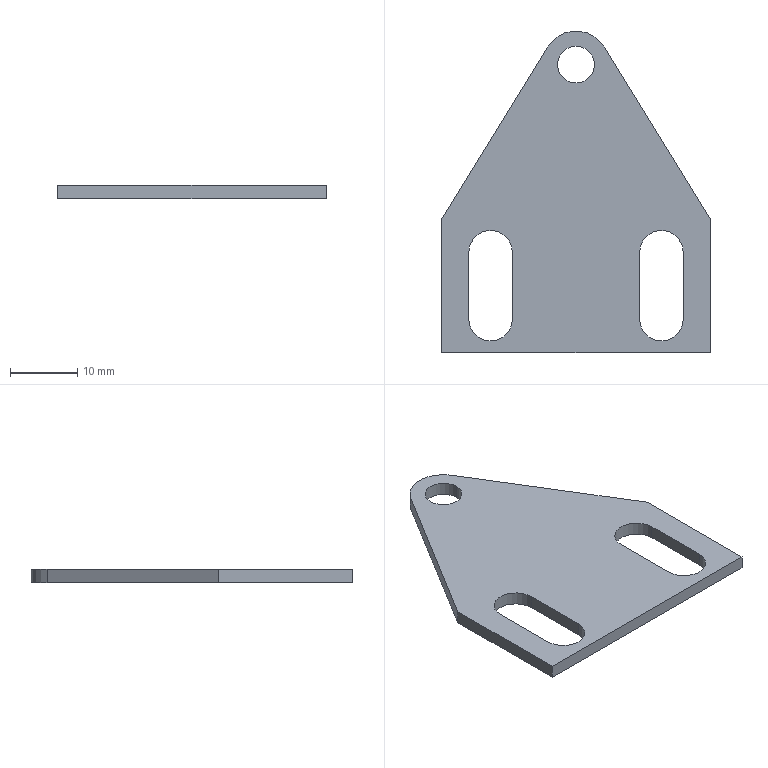Part | STEP file | Door catch sheet metal | 1 solid | 18 faces | box 40 x 48 x 2 mm | volume 2431 mm3 | plane 11 | cylinder 7 | commonest cylinder face diameters 6.5 x4 5.5 x2 10 x1
STEP:
#1=CARTESIAN_POINT('',(0.,0.,0.));
#2=DIRECTION('',(0.,0.,1.));
#3=DIRECTION('',(1.,0.,0.));
#4=AXIS2_PLACEMENT_3D('',#1,#2,#3);
#5=CARTESIAN_POINT('',(-2.75,19.,2.));
#6=VERTEX_POINT('',#5);
#7=CARTESIAN_POINT('',(-2.75,19.,0.));
#8=VERTEX_POINT('',#7);
#9=CARTESIAN_POINT('',(-2.75,19.,2.));
#10=DIRECTION('',(0.,0.,-1.));
#11=VECTOR('',#10,1.);
#12=LINE('',#9,#11);
#13=CARTESIAN_POINT('',(0.,19.,2.));
#14=DIRECTION('',(0.,0.,-1.));
#15=DIRECTION('',(-1.,0.,0.));
#16=AXIS2_PLACEMENT_3D('',#13,#14,#15);
#17=CYLINDRICAL_SURFACE('',#16,2.75);
#18=CARTESIAN_POINT('',(6.283,0.));
#19=DIRECTION('',(0.,1.));
#20=VECTOR('',#19,1.);
#21=LINE('',#18,#20);
#22=(GEOMETRIC_REPRESENTATION_CONTEXT(2)PARAMETRIC_REPRESENTATION_CONTEXT()REPRESENTATION_CONTEXT('',''));
#23=DEFINITIONAL_REPRESENTATION('',(#21),#22);
#24=PCURVE('',#17,#23);
#25=CARTESIAN_POINT('',(0.,19.,2.));
#26=DIRECTION('',(0.,0.,-1.));
#27=DIRECTION('',(-1.,0.,0.));
#28=AXIS2_PLACEMENT_3D('',#25,#26,#27);
#29=CYLINDRICAL_SURFACE('',#28,2.75);
#30=CARTESIAN_POINT('',(0.,0.));
#31=DIRECTION('',(0.,1.));
#32=VECTOR('',#31,1.);
#33=LINE('',#30,#32);
#34=(GEOMETRIC_REPRESENTATION_CONTEXT(2)PARAMETRIC_REPRESENTATION_CONTEXT()REPRESENTATION_CONTEXT('',''));
#35=DEFINITIONAL_REPRESENTATION('',(#33),#34);
#36=PCURVE('',#29,#35);
#37=SURFACE_CURVE('',#12,(#24,#36),.PCURVE_S1.);
#38=EDGE_CURVE('',#6,#8,#37,.T.);
#39=ORIENTED_EDGE('',*,*,#38,.T.);
#40=CARTESIAN_POINT('',(2.75,19.,0.));
#41=VERTEX_POINT('',#40);
#42=CARTESIAN_POINT('',(0.,19.,0.));
#43=DIRECTION('',(0.,0.,1.));
#44=DIRECTION('',(1.,0.,0.));
#45=AXIS2_PLACEMENT_3D('',#42,#43,#44);
#46=CIRCLE('',#45,2.75);
#47=CARTESIAN_POINT('',(9.425,2.));
#48=DIRECTION('',(-1.,0.));
#49=VECTOR('',#48,1.);
#50=LINE('',#47,#49);
#51=(GEOMETRIC_REPRESENTATION_CONTEXT(2)PARAMETRIC_REPRESENTATION_CONTEXT()REPRESENTATION_CONTEXT('',''));
#52=DEFINITIONAL_REPRESENTATION('',(#50),#51);
#53=PCURVE('',#17,#52);
#54=CARTESIAN_POINT('',(0.,0.,0.));
#55=DIRECTION('',(0.,0.,1.));
#56=DIRECTION('',(1.,0.,0.));
#57=AXIS2_PLACEMENT_3D('',#54,#55,#56);
#58=PLANE('',#57);
#59=CARTESIAN_POINT('',(0.,19.));
#60=DIRECTION('',(1.,0.));
#61=AXIS2_PLACEMENT_2D('',#59,#60);
#62=CIRCLE('',#61,2.75);
#63=(GEOMETRIC_REPRESENTATION_CONTEXT(2)PARAMETRIC_REPRESENTATION_CONTEXT()REPRESENTATION_CONTEXT('',''));
#64=DEFINITIONAL_REPRESENTATION('',(#62),#63);
#65=PCURVE('',#58,#64);
#66=SURFACE_CURVE('',#46,(#53,#65),.PCURVE_S1.);
#67=EDGE_CURVE('',#8,#41,#66,.T.);
#68=ORIENTED_EDGE('',*,*,#67,.T.);
#69=CARTESIAN_POINT('',(2.75,19.,2.));
#70=VERTEX_POINT('',#69);
#71=CARTESIAN_POINT('',(2.75,19.,2.));
#72=DIRECTION('',(0.,0.,-1.));
#73=VECTOR('',#72,1.);
#74=LINE('',#71,#73);
#75=CARTESIAN_POINT('',(3.142,0.));
#76=DIRECTION('',(0.,1.));
#77=VECTOR('',#76,1.);
#78=LINE('',#75,#77);
#79=(GEOMETRIC_REPRESENTATION_CONTEXT(2)PARAMETRIC_REPRESENTATION_CONTEXT()REPRESENTATION_CONTEXT('',''));
#80=DEFINITIONAL_REPRESENTATION('',(#78),#79);
#81=PCURVE('',#17,#80);
#82=CARTESIAN_POINT('',(3.142,0.));
#83=DIRECTION('',(0.,1.));
#84=VECTOR('',#83,1.);
#85=LINE('',#82,#84);
#86=(GEOMETRIC_REPRESENTATION_CONTEXT(2)PARAMETRIC_REPRESENTATION_CONTEXT()REPRESENTATION_CONTEXT('',''));
#87=DEFINITIONAL_REPRESENTATION('',(#85),#86);
#88=PCURVE('',#29,#87);
#89=SURFACE_CURVE('',#74,(#81,#88),.PCURVE_S1.);
#90=EDGE_CURVE('',#70,#41,#89,.T.);
#91=ORIENTED_EDGE('',*,*,#90,.F.);
#92=CARTESIAN_POINT('',(0.,19.,2.));
#93=DIRECTION('',(0.,0.,1.));
#94=DIRECTION('',(1.,0.,0.));
#95=AXIS2_PLACEMENT_3D('',#92,#93,#94);
#96=CIRCLE('',#95,2.75);
#97=CARTESIAN_POINT('',(9.425,0.));
#98=DIRECTION('',(-1.,0.));
#99=VECTOR('',#98,1.);
#100=LINE('',#97,#99);
#101=(GEOMETRIC_REPRESENTATION_CONTEXT(2)PARAMETRIC_REPRESENTATION_CONTEXT()REPRESENTATION_CONTEXT('',''));
#102=DEFINITIONAL_REPRESENTATION('',(#100),#101);
#103=PCURVE('',#17,#102);
#104=CARTESIAN_POINT('',(0.,0.,2.));
#105=DIRECTION('',(0.,0.,1.));
#106=DIRECTION('',(1.,0.,0.));
#107=AXIS2_PLACEMENT_3D('',#104,#105,#106);
#108=PLANE('',#107);
#109=CARTESIAN_POINT('',(0.,19.));
#110=DIRECTION('',(1.,0.));
#111=AXIS2_PLACEMENT_2D('',#109,#110);
#112=CIRCLE('',#111,2.75);
#113=(GEOMETRIC_REPRESENTATION_CONTEXT(2)PARAMETRIC_REPRESENTATION_CONTEXT()REPRESENTATION_CONTEXT('',''));
#114=DEFINITIONAL_REPRESENTATION('',(#112),#113);
#115=PCURVE('',#108,#114);
#116=SURFACE_CURVE('',#96,(#103,#115),.PCURVE_S1.);
#117=EDGE_CURVE('',#6,#70,#116,.T.);
#118=ORIENTED_EDGE('',*,*,#117,.F.);
#119=EDGE_LOOP('',(#39,#68,#91,#118));
#120=FACE_BOUND('',#119,.F.);
#121=ADVANCED_FACE('',(#120),#17,.F.);
#122=CARTESIAN_POINT('',(4.26,21.618,0.));
#123=VERTEX_POINT('',#122);
#124=CARTESIAN_POINT('',(20.,-4.,0.));
#125=VERTEX_POINT('',#124);
#126=CARTESIAN_POINT('',(12.735,7.825,0.));
#127=DIRECTION('',(0.5235,-0.852,0.));
#128=VECTOR('',#127,1.);
#129=LINE('',#126,#128);
#130=CARTESIAN_POINT('',(12.735,7.825,2.));
#131=DIRECTION('',(0.852,0.5235,0.));
#132=DIRECTION('',(-0.5235,0.852,0.));
#133=AXIS2_PLACEMENT_3D('',#130,#131,#132);
#134=PLANE('',#133);
#135=CARTESIAN_POINT('',(0.,-2.));
#136=DIRECTION('',(-1.,0.));
#137=VECTOR('',#136,1.);
#138=LINE('',#135,#137);
#139=(GEOMETRIC_REPRESENTATION_CONTEXT(2)PARAMETRIC_REPRESENTATION_CONTEXT()REPRESENTATION_CONTEXT('',''));
#140=DEFINITIONAL_REPRESENTATION('',(#138),#139);
#141=PCURVE('',#134,#140);
#142=CARTESIAN_POINT('',(12.735,7.825));
#143=DIRECTION('',(0.5235,-0.852));
#144=VECTOR('',#143,1.);
#145=LINE('',#142,#144);
#146=(GEOMETRIC_REPRESENTATION_CONTEXT(2)PARAMETRIC_REPRESENTATION_CONTEXT()REPRESENTATION_CONTEXT('',''));
#147=DEFINITIONAL_REPRESENTATION('',(#145),#146);
#148=PCURVE('',#58,#147);
#149=SURFACE_CURVE('',#129,(#141,#148),.PCURVE_S1.);
#150=EDGE_CURVE('',#123,#125,#149,.T.);
#151=ORIENTED_EDGE('',*,*,#150,.F.);
#152=CARTESIAN_POINT('',(4.26,21.618,2.));
#153=VERTEX_POINT('',#152);
#154=CARTESIAN_POINT('',(4.26,21.618,2.));
#155=DIRECTION('',(0.,0.,-1.));
#156=VECTOR('',#155,1.);
#157=LINE('',#154,#156);
#158=CARTESIAN_POINT('',(16.188,0.));
#159=DIRECTION('',(0.,-1.));
#160=VECTOR('',#159,1.);
#161=LINE('',#158,#160);
#162=(GEOMETRIC_REPRESENTATION_CONTEXT(2)PARAMETRIC_REPRESENTATION_CONTEXT()REPRESENTATION_CONTEXT('',''));
#163=DEFINITIONAL_REPRESENTATION('',(#161),#162);
#164=PCURVE('',#134,#163);
#165=CARTESIAN_POINT('',(0.,19.,2.));
#166=DIRECTION('',(0.,0.,-1.));
#167=DIRECTION('',(-1.,0.,0.));
#168=AXIS2_PLACEMENT_3D('',#165,#166,#167);
#169=CYLINDRICAL_SURFACE('',#168,5.);
#170=CARTESIAN_POINT('',(2.591,0.));
#171=DIRECTION('',(0.,1.));
#172=VECTOR('',#171,1.);
#173=LINE('',#170,#172);
#174=(GEOMETRIC_REPRESENTATION_CONTEXT(2)PARAMETRIC_REPRESENTATION_CONTEXT()REPRESENTATION_CONTEXT('',''));
#175=DEFINITIONAL_REPRESENTATION('',(#173),#174);
#176=PCURVE('',#169,#175);
#177=SURFACE_CURVE('',#157,(#164,#176),.PCURVE_S1.);
#178=EDGE_CURVE('',#153,#123,#177,.T.);
#179=ORIENTED_EDGE('',*,*,#178,.F.);
#180=CARTESIAN_POINT('',(20.,-4.,2.));
#181=VERTEX_POINT('',#180);
#182=CARTESIAN_POINT('',(12.735,7.825,2.));
#183=DIRECTION('',(0.5235,-0.852,0.));
#184=VECTOR('',#183,1.);
#185=LINE('',#182,#184);
#186=CARTESIAN_POINT('',(0.,0.));
#187=DIRECTION('',(-1.,0.));
#188=VECTOR('',#187,1.);
#189=LINE('',#186,#188);
#190=(GEOMETRIC_REPRESENTATION_CONTEXT(2)PARAMETRIC_REPRESENTATION_CONTEXT()REPRESENTATION_CONTEXT('',''));
#191=DEFINITIONAL_REPRESENTATION('',(#189),#190);
#192=PCURVE('',#134,#191);
#193=CARTESIAN_POINT('',(12.735,7.825));
#194=DIRECTION('',(0.5235,-0.852));
#195=VECTOR('',#194,1.);
#196=LINE('',#193,#195);
#197=(GEOMETRIC_REPRESENTATION_CONTEXT(2)PARAMETRIC_REPRESENTATION_CONTEXT()REPRESENTATION_CONTEXT('',''));
#198=DEFINITIONAL_REPRESENTATION('',(#196),#197);
#199=PCURVE('',#108,#198);
#200=SURFACE_CURVE('',#185,(#192,#199),.PCURVE_S1.);
#201=EDGE_CURVE('',#153,#181,#200,.T.);
#202=ORIENTED_EDGE('',*,*,#201,.T.);
#203=CARTESIAN_POINT('',(20.,-4.,2.));
#204=DIRECTION('',(0.,0.,-1.));
#205=VECTOR('',#204,1.);
#206=LINE('',#203,#205);
#207=CARTESIAN_POINT('',(-13.878,0.));
#208=DIRECTION('',(0.,-1.));
#209=VECTOR('',#208,1.);
#210=LINE('',#207,#209);
#211=(GEOMETRIC_REPRESENTATION_CONTEXT(2)PARAMETRIC_REPRESENTATION_CONTEXT()REPRESENTATION_CONTEXT('',''));
#212=DEFINITIONAL_REPRESENTATION('',(#210),#211);
#213=PCURVE('',#134,#212);
#214=CARTESIAN_POINT('',(20.,0.,2.));
#215=DIRECTION('',(1.,0.,0.));
#216=DIRECTION('',(0.,1.,0.));
#217=AXIS2_PLACEMENT_3D('',#214,#215,#216);
#218=PLANE('',#217);
#219=CARTESIAN_POINT('',(-4.,0.));
#220=DIRECTION('',(0.,-1.));
#221=VECTOR('',#220,1.);
#222=LINE('',#219,#221);
#223=(GEOMETRIC_REPRESENTATION_CONTEXT(2)PARAMETRIC_REPRESENTATION_CONTEXT()REPRESENTATION_CONTEXT('',''));
#224=DEFINITIONAL_REPRESENTATION('',(#222),#223);
#225=PCURVE('',#218,#224);
#226=SURFACE_CURVE('',#206,(#213,#225),.PCURVE_S1.);
#227=EDGE_CURVE('',#181,#125,#226,.T.);
#228=ORIENTED_EDGE('',*,*,#227,.T.);
#229=EDGE_LOOP('',(#151,#179,#202,#228));
#230=FACE_BOUND('',#229,.T.);
#231=ADVANCED_FACE('',(#230),#134,.T.);
#232=CARTESIAN_POINT('',(-4.26,21.618,0.));
#233=VERTEX_POINT('',#232);
#234=CARTESIAN_POINT('',(0.,19.,0.));
#235=DIRECTION('',(0.,0.,1.));
#236=DIRECTION('',(1.,0.,0.));
#237=AXIS2_PLACEMENT_3D('',#234,#235,#236);
#238=CIRCLE('',#237,5.);
#239=CARTESIAN_POINT('',(3.142,2.));
#240=DIRECTION('',(-1.,0.));
#241=VECTOR('',#240,1.);
#242=LINE('',#239,#241);
#243=(GEOMETRIC_REPRESENTATION_CONTEXT(2)PARAMETRIC_REPRESENTATION_CONTEXT()REPRESENTATION_CONTEXT('',''));
#244=DEFINITIONAL_REPRESENTATION('',(#242),#243);
#245=PCURVE('',#169,#244);
#246=CARTESIAN_POINT('',(0.,19.));
#247=DIRECTION('',(1.,0.));
#248=AXIS2_PLACEMENT_2D('',#246,#247);
#249=CIRCLE('',#248,5.);
#250=(GEOMETRIC_REPRESENTATION_CONTEXT(2)PARAMETRIC_REPRESENTATION_CONTEXT()REPRESENTATION_CONTEXT('',''));
#251=DEFINITIONAL_REPRESENTATION('',(#249),#250);
#252=PCURVE('',#58,#251);
#253=SURFACE_CURVE('',#238,(#245,#252),.PCURVE_S1.);
#254=EDGE_CURVE('',#123,#233,#253,.T.);
#255=ORIENTED_EDGE('',*,*,#254,.T.);
#256=CARTESIAN_POINT('',(-4.26,21.618,2.));
#257=VERTEX_POINT('',#256);
#258=CARTESIAN_POINT('',(-4.26,21.618,2.));
#259=DIRECTION('',(0.,0.,-1.));
#260=VECTOR('',#259,1.);
#261=LINE('',#258,#260);
#262=CARTESIAN_POINT('',(0.551,0.));
#263=DIRECTION('',(0.,1.));
#264=VECTOR('',#263,1.);
#265=LINE('',#262,#264);
#266=(GEOMETRIC_REPRESENTATION_CONTEXT(2)PARAMETRIC_REPRESENTATION_CONTEXT()REPRESENTATION_CONTEXT('',''));
#267=DEFINITIONAL_REPRESENTATION('',(#265),#266);
#268=PCURVE('',#169,#267);
#269=CARTESIAN_POINT('',(-12.735,7.825,2.));
#270=DIRECTION('',(0.852,-0.5235,0.));
#271=DIRECTION('',(0.5235,0.852,0.));
#272=AXIS2_PLACEMENT_3D('',#269,#270,#271);
#273=PLANE('',#272);
#274=CARTESIAN_POINT('',(16.188,0.));
#275=DIRECTION('',(0.,-1.));
#276=VECTOR('',#275,1.);
#277=LINE('',#274,#276);
#278=(GEOMETRIC_REPRESENTATION_CONTEXT(2)PARAMETRIC_REPRESENTATION_CONTEXT()REPRESENTATION_CONTEXT('',''));
#279=DEFINITIONAL_REPRESENTATION('',(#277),#278);
#280=PCURVE('',#273,#279);
#281=SURFACE_CURVE('',#261,(#268,#280),.PCURVE_S1.);
#282=EDGE_CURVE('',#257,#233,#281,.T.);
#283=ORIENTED_EDGE('',*,*,#282,.F.);
#284=CARTESIAN_POINT('',(0.,19.,2.));
#285=DIRECTION('',(0.,0.,1.));
#286=DIRECTION('',(1.,0.,0.));
#287=AXIS2_PLACEMENT_3D('',#284,#285,#286);
#288=CIRCLE('',#287,5.);
#289=CARTESIAN_POINT('',(3.142,0.));
#290=DIRECTION('',(-1.,0.));
#291=VECTOR('',#290,1.);
#292=LINE('',#289,#291);
#293=(GEOMETRIC_REPRESENTATION_CONTEXT(2)PARAMETRIC_REPRESENTATION_CONTEXT()REPRESENTATION_CONTEXT('',''));
#294=DEFINITIONAL_REPRESENTATION('',(#292),#293);
#295=PCURVE('',#169,#294);
#296=CARTESIAN_POINT('',(0.,19.));
#297=DIRECTION('',(1.,0.));
#298=AXIS2_PLACEMENT_2D('',#296,#297);
#299=CIRCLE('',#298,5.);
#300=(GEOMETRIC_REPRESENTATION_CONTEXT(2)PARAMETRIC_REPRESENTATION_CONTEXT()REPRESENTATION_CONTEXT('',''));
#301=DEFINITIONAL_REPRESENTATION('',(#299),#300);
#302=PCURVE('',#108,#301);
#303=SURFACE_CURVE('',#288,(#295,#302),.PCURVE_S1.);
#304=EDGE_CURVE('',#153,#257,#303,.T.);
#305=ORIENTED_EDGE('',*,*,#304,.F.);
#306=ORIENTED_EDGE('',*,*,#178,.T.);
#307=EDGE_LOOP('',(#255,#283,#305,#306));
#308=FACE_BOUND('',#307,.T.);
#309=ADVANCED_FACE('',(#308),#169,.T.);
#310=CARTESIAN_POINT('',(-20.,-4.,0.));
#311=VERTEX_POINT('',#310);
#312=CARTESIAN_POINT('',(-12.735,7.825,0.));
#313=DIRECTION('',(-0.5235,-0.852,0.));
#314=VECTOR('',#313,1.);
#315=LINE('',#312,#314);
#316=CARTESIAN_POINT('',(0.,-2.));
#317=DIRECTION('',(-1.,0.));
#318=VECTOR('',#317,1.);
#319=LINE('',#316,#318);
#320=(GEOMETRIC_REPRESENTATION_CONTEXT(2)PARAMETRIC_REPRESENTATION_CONTEXT()REPRESENTATION_CONTEXT('',''));
#321=DEFINITIONAL_REPRESENTATION('',(#319),#320);
#322=PCURVE('',#273,#321);
#323=CARTESIAN_POINT('',(-12.735,7.825));
#324=DIRECTION('',(-0.5235,-0.852));
#325=VECTOR('',#324,1.);
#326=LINE('',#323,#325);
#327=(GEOMETRIC_REPRESENTATION_CONTEXT(2)PARAMETRIC_REPRESENTATION_CONTEXT()REPRESENTATION_CONTEXT('',''));
#328=DEFINITIONAL_REPRESENTATION('',(#326),#327);
#329=PCURVE('',#58,#328);
#330=SURFACE_CURVE('',#315,(#322,#329),.PCURVE_S1.);
#331=EDGE_CURVE('',#233,#311,#330,.T.);
#332=ORIENTED_EDGE('',*,*,#331,.T.);
#333=CARTESIAN_POINT('',(-20.,-4.,2.));
#334=VERTEX_POINT('',#333);
#335=CARTESIAN_POINT('',(-20.,-4.,2.));
#336=DIRECTION('',(0.,0.,-1.));
#337=VECTOR('',#336,1.);
#338=LINE('',#335,#337);
#339=CARTESIAN_POINT('',(-13.878,0.));
#340=DIRECTION('',(0.,-1.));
#341=VECTOR('',#340,1.);
#342=LINE('',#339,#341);
#343=(GEOMETRIC_REPRESENTATION_CONTEXT(2)PARAMETRIC_REPRESENTATION_CONTEXT()REPRESENTATION_CONTEXT('',''));
#344=DEFINITIONAL_REPRESENTATION('',(#342),#343);
#345=PCURVE('',#273,#344);
#346=CARTESIAN_POINT('',(-20.,0.,2.));
#347=DIRECTION('',(1.,0.,0.));
#348=DIRECTION('',(0.,1.,0.));
#349=AXIS2_PLACEMENT_3D('',#346,#347,#348);
#350=PLANE('',#349);
#351=CARTESIAN_POINT('',(-4.,0.));
#352=DIRECTION('',(0.,-1.));
#353=VECTOR('',#352,1.);
#354=LINE('',#351,#353);
#355=(GEOMETRIC_REPRESENTATION_CONTEXT(2)PARAMETRIC_REPRESENTATION_CONTEXT()REPRESENTATION_CONTEXT('',''));
#356=DEFINITIONAL_REPRESENTATION('',(#354),#355);
#357=PCURVE('',#350,#356);
#358=SURFACE_CURVE('',#338,(#345,#357),.PCURVE_S1.);
#359=EDGE_CURVE('',#334,#311,#358,.T.);
#360=ORIENTED_EDGE('',*,*,#359,.F.);
#361=CARTESIAN_POINT('',(-12.735,7.825,2.));
#362=DIRECTION('',(-0.5235,-0.852,0.));
#363=VECTOR('',#362,1.);
#364=LINE('',#361,#363);
#365=CARTESIAN_POINT('',(0.,0.));
#366=DIRECTION('',(-1.,0.));
#367=VECTOR('',#366,1.);
#368=LINE('',#365,#367);
#369=(GEOMETRIC_REPRESENTATION_CONTEXT(2)PARAMETRIC_REPRESENTATION_CONTEXT()REPRESENTATION_CONTEXT('',''));
#370=DEFINITIONAL_REPRESENTATION('',(#368),#369);
#371=PCURVE('',#273,#370);
#372=CARTESIAN_POINT('',(-12.735,7.825));
#373=DIRECTION('',(-0.5235,-0.852));
#374=VECTOR('',#373,1.);
#375=LINE('',#372,#374);
#376=(GEOMETRIC_REPRESENTATION_CONTEXT(2)PARAMETRIC_REPRESENTATION_CONTEXT()REPRESENTATION_CONTEXT('',''));
#377=DEFINITIONAL_REPRESENTATION('',(#375),#376);
#378=PCURVE('',#108,#377);
#379=SURFACE_CURVE('',#364,(#371,#378),.PCURVE_S1.);
#380=EDGE_CURVE('',#257,#334,#379,.T.);
#381=ORIENTED_EDGE('',*,*,#380,.F.);
#382=ORIENTED_EDGE('',*,*,#282,.T.);
#383=EDGE_LOOP('',(#332,#360,#381,#382));
#384=FACE_BOUND('',#383,.T.);
#385=ADVANCED_FACE('',(#384),#273,.F.);
#386=CARTESIAN_POINT('',(-20.,-24.,0.));
#387=VERTEX_POINT('',#386);
#388=CARTESIAN_POINT('',(-20.,0.,0.));
#389=DIRECTION('',(0.,-1.,0.));
#390=VECTOR('',#389,1.);
#391=LINE('',#388,#390);
#392=CARTESIAN_POINT('',(0.,-2.));
#393=DIRECTION('',(-1.,0.));
#394=VECTOR('',#393,1.);
#395=LINE('',#392,#394);
#396=(GEOMETRIC_REPRESENTATION_CONTEXT(2)PARAMETRIC_REPRESENTATION_CONTEXT()REPRESENTATION_CONTEXT('',''));
#397=DEFINITIONAL_REPRESENTATION('',(#395),#396);
#398=PCURVE('',#350,#397);
#399=CARTESIAN_POINT('',(-20.,0.));
#400=DIRECTION('',(0.,-1.));
#401=VECTOR('',#400,1.);
#402=LINE('',#399,#401);
#403=(GEOMETRIC_REPRESENTATION_CONTEXT(2)PARAMETRIC_REPRESENTATION_CONTEXT()REPRESENTATION_CONTEXT('',''));
#404=DEFINITIONAL_REPRESENTATION('',(#402),#403);
#405=PCURVE('',#58,#404);
#406=SURFACE_CURVE('',#391,(#398,#405),.PCURVE_S1.);
#407=EDGE_CURVE('',#311,#387,#406,.T.);
#408=ORIENTED_EDGE('',*,*,#407,.T.);
#409=CARTESIAN_POINT('',(-20.,-24.,2.));
#410=VERTEX_POINT('',#409);
#411=CARTESIAN_POINT('',(-20.,-24.,2.));
#412=DIRECTION('',(0.,0.,-1.));
#413=VECTOR('',#412,1.);
#414=LINE('',#411,#413);
#415=CARTESIAN_POINT('',(-24.,0.));
#416=DIRECTION('',(0.,-1.));
#417=VECTOR('',#416,1.);
#418=LINE('',#415,#417);
#419=(GEOMETRIC_REPRESENTATION_CONTEXT(2)PARAMETRIC_REPRESENTATION_CONTEXT()REPRESENTATION_CONTEXT('',''));
#420=DEFINITIONAL_REPRESENTATION('',(#418),#419);
#421=PCURVE('',#350,#420);
#422=CARTESIAN_POINT('',(0.,-24.,2.));
#423=DIRECTION('',(0.,1.,0.));
#424=DIRECTION('',(0.,0.,1.));
#425=AXIS2_PLACEMENT_3D('',#422,#423,#424);
#426=PLANE('',#425);
#427=CARTESIAN_POINT('',(0.,-20.));
#428=DIRECTION('',(-1.,0.));
#429=VECTOR('',#428,1.);
#430=LINE('',#427,#429);
#431=(GEOMETRIC_REPRESENTATION_CONTEXT(2)PARAMETRIC_REPRESENTATION_CONTEXT()REPRESENTATION_CONTEXT('',''));
#432=DEFINITIONAL_REPRESENTATION('',(#430),#431);
#433=PCURVE('',#426,#432);
#434=SURFACE_CURVE('',#414,(#421,#433),.PCURVE_S1.);
#435=EDGE_CURVE('',#410,#387,#434,.T.);
#436=ORIENTED_EDGE('',*,*,#435,.F.);
#437=CARTESIAN_POINT('',(-20.,0.,2.));
#438=DIRECTION('',(0.,-1.,0.));
#439=VECTOR('',#438,1.);
#440=LINE('',#437,#439);
#441=CARTESIAN_POINT('',(0.,0.));
#442=DIRECTION('',(-1.,0.));
#443=VECTOR('',#442,1.);
#444=LINE('',#441,#443);
#445=(GEOMETRIC_REPRESENTATION_CONTEXT(2)PARAMETRIC_REPRESENTATION_CONTEXT()REPRESENTATION_CONTEXT('',''));
#446=DEFINITIONAL_REPRESENTATION('',(#444),#445);
#447=PCURVE('',#350,#446);
#448=CARTESIAN_POINT('',(-20.,0.));
#449=DIRECTION('',(0.,-1.));
#450=VECTOR('',#449,1.);
#451=LINE('',#448,#450);
#452=(GEOMETRIC_REPRESENTATION_CONTEXT(2)PARAMETRIC_REPRESENTATION_CONTEXT()REPRESENTATION_CONTEXT('',''));
#453=DEFINITIONAL_REPRESENTATION('',(#451),#452);
#454=PCURVE('',#108,#453);
#455=SURFACE_CURVE('',#440,(#447,#454),.PCURVE_S1.);
#456=EDGE_CURVE('',#334,#410,#455,.T.);
#457=ORIENTED_EDGE('',*,*,#456,.F.);
#458=ORIENTED_EDGE('',*,*,#359,.T.);
#459=EDGE_LOOP('',(#408,#436,#457,#458));
#460=FACE_BOUND('',#459,.T.);
#461=ADVANCED_FACE('',(#460),#350,.F.);
#462=CARTESIAN_POINT('',(20.,-24.,0.));
#463=VERTEX_POINT('',#462);
#464=CARTESIAN_POINT('',(0.,-24.,0.));
#465=DIRECTION('',(1.,0.,0.));
#466=VECTOR('',#465,1.);
#467=LINE('',#464,#466);
#468=CARTESIAN_POINT('',(-2.,0.));
#469=DIRECTION('',(0.,1.));
#470=VECTOR('',#469,1.);
#471=LINE('',#468,#470);
#472=(GEOMETRIC_REPRESENTATION_CONTEXT(2)PARAMETRIC_REPRESENTATION_CONTEXT()REPRESENTATION_CONTEXT('',''));
#473=DEFINITIONAL_REPRESENTATION('',(#471),#472);
#474=PCURVE('',#426,#473);
#475=CARTESIAN_POINT('',(0.,-24.));
#476=DIRECTION('',(1.,0.));
#477=VECTOR('',#476,1.);
#478=LINE('',#475,#477);
#479=(GEOMETRIC_REPRESENTATION_CONTEXT(2)PARAMETRIC_REPRESENTATION_CONTEXT()REPRESENTATION_CONTEXT('',''));
#480=DEFINITIONAL_REPRESENTATION('',(#478),#479);
#481=PCURVE('',#58,#480);
#482=SURFACE_CURVE('',#467,(#474,#481),.PCURVE_S1.);
#483=EDGE_CURVE('',#387,#463,#482,.T.);
#484=ORIENTED_EDGE('',*,*,#483,.T.);
#485=CARTESIAN_POINT('',(20.,-24.,2.));
#486=VERTEX_POINT('',#485);
#487=CARTESIAN_POINT('',(20.,-24.,2.));
#488=DIRECTION('',(0.,0.,-1.));
#489=VECTOR('',#488,1.);
#490=LINE('',#487,#489);
#491=CARTESIAN_POINT('',(0.,20.));
#492=DIRECTION('',(-1.,0.));
#493=VECTOR('',#492,1.);
#494=LINE('',#491,#493);
#495=(GEOMETRIC_REPRESENTATION_CONTEXT(2)PARAMETRIC_REPRESENTATION_CONTEXT()REPRESENTATION_CONTEXT('',''));
#496=DEFINITIONAL_REPRESENTATION('',(#494),#495);
#497=PCURVE('',#426,#496);
#498=CARTESIAN_POINT('',(-24.,0.));
#499=DIRECTION('',(0.,-1.));
#500=VECTOR('',#499,1.);
#501=LINE('',#498,#500);
#502=(GEOMETRIC_REPRESENTATION_CONTEXT(2)PARAMETRIC_REPRESENTATION_CONTEXT()REPRESENTATION_CONTEXT('',''));
#503=DEFINITIONAL_REPRESENTATION('',(#501),#502);
#504=PCURVE('',#218,#503);
#505=SURFACE_CURVE('',#490,(#497,#504),.PCURVE_S1.);
#506=EDGE_CURVE('',#486,#463,#505,.T.);
#507=ORIENTED_EDGE('',*,*,#506,.F.);
#508=CARTESIAN_POINT('',(0.,-24.,2.));
#509=DIRECTION('',(1.,0.,0.));
#510=VECTOR('',#509,1.);
#511=LINE('',#508,#510);
#512=CARTESIAN_POINT('',(0.,0.));
#513=DIRECTION('',(0.,1.));
#514=VECTOR('',#513,1.);
#515=LINE('',#512,#514);
#516=(GEOMETRIC_REPRESENTATION_CONTEXT(2)PARAMETRIC_REPRESENTATION_CONTEXT()REPRESENTATION_CONTEXT('',''));
#517=DEFINITIONAL_REPRESENTATION('',(#515),#516);
#518=PCURVE('',#426,#517);
#519=CARTESIAN_POINT('',(0.,-24.));
#520=DIRECTION('',(1.,0.));
#521=VECTOR('',#520,1.);
#522=LINE('',#519,#521);
#523=(GEOMETRIC_REPRESENTATION_CONTEXT(2)PARAMETRIC_REPRESENTATION_CONTEXT()REPRESENTATION_CONTEXT('',''));
#524=DEFINITIONAL_REPRESENTATION('',(#522),#523);
#525=PCURVE('',#108,#524);
#526=SURFACE_CURVE('',#511,(#518,#525),.PCURVE_S1.);
#527=EDGE_CURVE('',#410,#486,#526,.T.);
#528=ORIENTED_EDGE('',*,*,#527,.F.);
#529=ORIENTED_EDGE('',*,*,#435,.T.);
#530=EDGE_LOOP('',(#484,#507,#528,#529));
#531=FACE_BOUND('',#530,.T.);
#532=ADVANCED_FACE('',(#531),#426,.F.);
#533=CARTESIAN_POINT('',(-9.5,-19.,2.));
#534=VERTEX_POINT('',#533);
#535=CARTESIAN_POINT('',(-9.5,-19.,0.));
#536=VERTEX_POINT('',#535);
#537=CARTESIAN_POINT('',(-9.5,-19.,2.));
#538=DIRECTION('',(0.,0.,-1.));
#539=VECTOR('',#538,1.);
#540=LINE('',#537,#539);
#541=CARTESIAN_POINT('',(-12.75,-19.,2.));
#542=DIRECTION('',(0.,0.,-1.));
#543=DIRECTION('',(-1.,0.,0.));
#544=AXIS2_PLACEMENT_3D('',#541,#542,#543);
#545=CYLINDRICAL_SURFACE('',#544,3.25);
#546=CARTESIAN_POINT('',(3.142,0.));
#547=DIRECTION('',(0.,1.));
#548=VECTOR('',#547,1.);
#549=LINE('',#546,#548);
#550=(GEOMETRIC_REPRESENTATION_CONTEXT(2)PARAMETRIC_REPRESENTATION_CONTEXT()REPRESENTATION_CONTEXT('',''));
#551=DEFINITIONAL_REPRESENTATION('',(#549),#550);
#552=PCURVE('',#545,#551);
#553=CARTESIAN_POINT('',(-9.5,0.,2.));
#554=DIRECTION('',(1.,0.,0.));
#555=DIRECTION('',(0.,0.,-1.));
#556=AXIS2_PLACEMENT_3D('',#553,#554,#555);
#557=PLANE('',#556);
#558=CARTESIAN_POINT('',(0.,-19.));
#559=DIRECTION('',(1.,0.));
#560=VECTOR('',#559,1.);
#561=LINE('',#558,#560);
#562=(GEOMETRIC_REPRESENTATION_CONTEXT(2)PARAMETRIC_REPRESENTATION_CONTEXT()REPRESENTATION_CONTEXT('',''));
#563=DEFINITIONAL_REPRESENTATION('',(#561),#562);
#564=PCURVE('',#557,#563);
#565=SURFACE_CURVE('',#540,(#552,#564),.PCURVE_S1.);
#566=EDGE_CURVE('',#534,#536,#565,.T.);
#567=ORIENTED_EDGE('',*,*,#566,.F.);
#568=CARTESIAN_POINT('',(-16.,-19.,2.));
#569=VERTEX_POINT('',#568);
#570=CARTESIAN_POINT('',(-12.75,-19.,2.));
#571=DIRECTION('',(0.,0.,1.));
#572=DIRECTION('',(1.,0.,0.));
#573=AXIS2_PLACEMENT_3D('',#570,#571,#572);
#574=CIRCLE('',#573,3.25);
#575=CARTESIAN_POINT('',(9.425,0.));
#576=DIRECTION('',(-1.,0.));
#577=VECTOR('',#576,1.);
#578=LINE('',#575,#577);
#579=(GEOMETRIC_REPRESENTATION_CONTEXT(2)PARAMETRIC_REPRESENTATION_CONTEXT()REPRESENTATION_CONTEXT('',''));
#580=DEFINITIONAL_REPRESENTATION('',(#578),#579);
#581=PCURVE('',#545,#580);
#582=CARTESIAN_POINT('',(-12.75,-19.));
#583=DIRECTION('',(1.,0.));
#584=AXIS2_PLACEMENT_2D('',#582,#583);
#585=CIRCLE('',#584,3.25);
#586=(GEOMETRIC_REPRESENTATION_CONTEXT(2)PARAMETRIC_REPRESENTATION_CONTEXT()REPRESENTATION_CONTEXT('',''));
#587=DEFINITIONAL_REPRESENTATION('',(#585),#586);
#588=PCURVE('',#108,#587);
#589=SURFACE_CURVE('',#574,(#581,#588),.PCURVE_S1.);
#590=EDGE_CURVE('',#569,#534,#589,.T.);
#591=ORIENTED_EDGE('',*,*,#590,.F.);
#592=CARTESIAN_POINT('',(-16.,-19.,0.));
#593=VERTEX_POINT('',#592);
#594=CARTESIAN_POINT('',(-16.,-19.,2.));
#595=DIRECTION('',(0.,0.,-1.));
#596=VECTOR('',#595,1.);
#597=LINE('',#594,#596);
#598=CARTESIAN_POINT('',(6.283,0.));
#599=DIRECTION('',(0.,1.));
#600=VECTOR('',#599,1.);
#601=LINE('',#598,#600);
#602=(GEOMETRIC_REPRESENTATION_CONTEXT(2)PARAMETRIC_REPRESENTATION_CONTEXT()REPRESENTATION_CONTEXT('',''));
#603=DEFINITIONAL_REPRESENTATION('',(#601),#602);
#604=PCURVE('',#545,#603);
#605=CARTESIAN_POINT('',(-16.,0.,2.));
#606=DIRECTION('',(1.,0.,0.));
#607=DIRECTION('',(0.,0.,-1.));
#608=AXIS2_PLACEMENT_3D('',#605,#606,#607);
#609=PLANE('',#608);
#610=CARTESIAN_POINT('',(0.,-19.));
#611=DIRECTION('',(1.,0.));
#612=VECTOR('',#611,1.);
#613=LINE('',#610,#612);
#614=(GEOMETRIC_REPRESENTATION_CONTEXT(2)PARAMETRIC_REPRESENTATION_CONTEXT()REPRESENTATION_CONTEXT('',''));
#615=DEFINITIONAL_REPRESENTATION('',(#613),#614);
#616=PCURVE('',#609,#615);
#617=SURFACE_CURVE('',#597,(#604,#616),.PCURVE_S1.);
#618=EDGE_CURVE('',#569,#593,#617,.T.);
#619=ORIENTED_EDGE('',*,*,#618,.T.);
#620=CARTESIAN_POINT('',(-12.75,-19.,0.));
#621=DIRECTION('',(0.,0.,1.));
#622=DIRECTION('',(1.,0.,0.));
#623=AXIS2_PLACEMENT_3D('',#620,#621,#622);
#624=CIRCLE('',#623,3.25);
#625=CARTESIAN_POINT('',(9.425,2.));
#626=DIRECTION('',(-1.,0.));
#627=VECTOR('',#626,1.);
#628=LINE('',#625,#627);
#629=(GEOMETRIC_REPRESENTATION_CONTEXT(2)PARAMETRIC_REPRESENTATION_CONTEXT()REPRESENTATION_CONTEXT('',''));
#630=DEFINITIONAL_REPRESENTATION('',(#628),#629);
#631=PCURVE('',#545,#630);
#632=CARTESIAN_POINT('',(-12.75,-19.));
#633=DIRECTION('',(1.,0.));
#634=AXIS2_PLACEMENT_2D('',#632,#633);
#635=CIRCLE('',#634,3.25);
#636=(GEOMETRIC_REPRESENTATION_CONTEXT(2)PARAMETRIC_REPRESENTATION_CONTEXT()REPRESENTATION_CONTEXT('',''));
#637=DEFINITIONAL_REPRESENTATION('',(#635),#636);
#638=PCURVE('',#58,#637);
#639=SURFACE_CURVE('',#624,(#631,#638),.PCURVE_S1.);
#640=EDGE_CURVE('',#593,#536,#639,.T.);
#641=ORIENTED_EDGE('',*,*,#640,.T.);
#642=EDGE_LOOP('',(#567,#591,#619,#641));
#643=FACE_BOUND('',#642,.F.);
#644=ADVANCED_FACE('',(#643),#545,.F.);
#645=CARTESIAN_POINT('',(-16.,-9.,0.));
#646=VERTEX_POINT('',#645);
#647=CARTESIAN_POINT('',(-16.,0.,0.));
#648=DIRECTION('',(0.,-1.,0.));
#649=VECTOR('',#648,1.);
#650=LINE('',#647,#649);
#651=CARTESIAN_POINT('',(2.,0.));
#652=DIRECTION('',(0.,-1.));
#653=VECTOR('',#652,1.);
#654=LINE('',#651,#653);
#655=(GEOMETRIC_REPRESENTATION_CONTEXT(2)PARAMETRIC_REPRESENTATION_CONTEXT()REPRESENTATION_CONTEXT('',''));
#656=DEFINITIONAL_REPRESENTATION('',(#654),#655);
#657=PCURVE('',#609,#656);
#658=CARTESIAN_POINT('',(-16.,0.));
#659=DIRECTION('',(0.,-1.));
#660=VECTOR('',#659,1.);
#661=LINE('',#658,#660);
#662=(GEOMETRIC_REPRESENTATION_CONTEXT(2)PARAMETRIC_REPRESENTATION_CONTEXT()REPRESENTATION_CONTEXT('',''));
#663=DEFINITIONAL_REPRESENTATION('',(#661),#662);
#664=PCURVE('',#58,#663);
#665=SURFACE_CURVE('',#650,(#657,#664),.PCURVE_S1.);
#666=EDGE_CURVE('',#646,#593,#665,.T.);
#667=ORIENTED_EDGE('',*,*,#666,.F.);
#668=CARTESIAN_POINT('',(-16.,-9.,2.));
#669=VERTEX_POINT('',#668);
#670=CARTESIAN_POINT('',(-16.,-9.,2.));
#671=DIRECTION('',(0.,0.,-1.));
#672=VECTOR('',#671,1.);
#673=LINE('',#670,#672);
#674=CARTESIAN_POINT('',(0.,-9.));
#675=DIRECTION('',(1.,0.));
#676=VECTOR('',#675,1.);
#677=LINE('',#674,#676);
#678=(GEOMETRIC_REPRESENTATION_CONTEXT(2)PARAMETRIC_REPRESENTATION_CONTEXT()REPRESENTATION_CONTEXT('',''));
#679=DEFINITIONAL_REPRESENTATION('',(#677),#678);
#680=PCURVE('',#609,#679);
#681=CARTESIAN_POINT('',(-12.75,-9.,2.));
#682=DIRECTION('',(0.,0.,-1.));
#683=DIRECTION('',(-1.,0.,0.));
#684=AXIS2_PLACEMENT_3D('',#681,#682,#683);
#685=CYLINDRICAL_SURFACE('',#684,3.25);
#686=CARTESIAN_POINT('',(0.,0.));
#687=DIRECTION('',(0.,1.));
#688=VECTOR('',#687,1.);
#689=LINE('',#686,#688);
#690=(GEOMETRIC_REPRESENTATION_CONTEXT(2)PARAMETRIC_REPRESENTATION_CONTEXT()REPRESENTATION_CONTEXT('',''));
#691=DEFINITIONAL_REPRESENTATION('',(#689),#690);
#692=PCURVE('',#685,#691);
#693=SURFACE_CURVE('',#673,(#680,#692),.PCURVE_S1.);
#694=EDGE_CURVE('',#669,#646,#693,.T.);
#695=ORIENTED_EDGE('',*,*,#694,.F.);
#696=CARTESIAN_POINT('',(-16.,0.,2.));
#697=DIRECTION('',(0.,-1.,0.));
#698=VECTOR('',#697,1.);
#699=LINE('',#696,#698);
#700=CARTESIAN_POINT('',(0.,0.));
#701=DIRECTION('',(0.,-1.));
#702=VECTOR('',#701,1.);
#703=LINE('',#700,#702);
#704=(GEOMETRIC_REPRESENTATION_CONTEXT(2)PARAMETRIC_REPRESENTATION_CONTEXT()REPRESENTATION_CONTEXT('',''));
#705=DEFINITIONAL_REPRESENTATION('',(#703),#704);
#706=PCURVE('',#609,#705);
#707=CARTESIAN_POINT('',(-16.,0.));
#708=DIRECTION('',(0.,-1.));
#709=VECTOR('',#708,1.);
#710=LINE('',#707,#709);
#711=(GEOMETRIC_REPRESENTATION_CONTEXT(2)PARAMETRIC_REPRESENTATION_CONTEXT()REPRESENTATION_CONTEXT('',''));
#712=DEFINITIONAL_REPRESENTATION('',(#710),#711);
#713=PCURVE('',#108,#712);
#714=SURFACE_CURVE('',#699,(#706,#713),.PCURVE_S1.);
#715=EDGE_CURVE('',#669,#569,#714,.T.);
#716=ORIENTED_EDGE('',*,*,#715,.T.);
#717=ORIENTED_EDGE('',*,*,#618,.T.);
#718=EDGE_LOOP('',(#667,#695,#716,#717));
#719=FACE_BOUND('',#718,.T.);
#720=ADVANCED_FACE('',(#719),#609,.T.);
#721=ORIENTED_EDGE('',*,*,#694,.F.);
#722=CARTESIAN_POINT('',(-9.5,-9.,2.));
#723=VERTEX_POINT('',#722);
#724=CARTESIAN_POINT('',(-12.75,-9.,2.));
#725=DIRECTION('',(0.,0.,1.));
#726=DIRECTION('',(1.,0.,0.));
#727=AXIS2_PLACEMENT_3D('',#724,#725,#726);
#728=CIRCLE('',#727,3.25);
#729=CARTESIAN_POINT('',(3.142,0.));
#730=DIRECTION('',(-1.,0.));
#731=VECTOR('',#730,1.);
#732=LINE('',#729,#731);
#733=(GEOMETRIC_REPRESENTATION_CONTEXT(2)PARAMETRIC_REPRESENTATION_CONTEXT()REPRESENTATION_CONTEXT('',''));
#734=DEFINITIONAL_REPRESENTATION('',(#732),#733);
#735=PCURVE('',#685,#734);
#736=CARTESIAN_POINT('',(-12.75,-9.));
#737=DIRECTION('',(1.,0.));
#738=AXIS2_PLACEMENT_2D('',#736,#737);
#739=CIRCLE('',#738,3.25);
#740=(GEOMETRIC_REPRESENTATION_CONTEXT(2)PARAMETRIC_REPRESENTATION_CONTEXT()REPRESENTATION_CONTEXT('',''));
#741=DEFINITIONAL_REPRESENTATION('',(#739),#740);
#742=PCURVE('',#108,#741);
#743=SURFACE_CURVE('',#728,(#735,#742),.PCURVE_S1.);
#744=EDGE_CURVE('',#723,#669,#743,.T.);
#745=ORIENTED_EDGE('',*,*,#744,.F.);
#746=CARTESIAN_POINT('',(-9.5,-9.,0.));
#747=VERTEX_POINT('',#746);
#748=CARTESIAN_POINT('',(-9.5,-9.,2.));
#749=DIRECTION('',(0.,0.,-1.));
#750=VECTOR('',#749,1.);
#751=LINE('',#748,#750);
#752=CARTESIAN_POINT('',(3.142,0.));
#753=DIRECTION('',(0.,1.));
#754=VECTOR('',#753,1.);
#755=LINE('',#752,#754);
#756=(GEOMETRIC_REPRESENTATION_CONTEXT(2)PARAMETRIC_REPRESENTATION_CONTEXT()REPRESENTATION_CONTEXT('',''));
#757=DEFINITIONAL_REPRESENTATION('',(#755),#756);
#758=PCURVE('',#685,#757);
#759=CARTESIAN_POINT('',(0.,-9.));
#760=DIRECTION('',(1.,0.));
#761=VECTOR('',#760,1.);
#762=LINE('',#759,#761);
#763=(GEOMETRIC_REPRESENTATION_CONTEXT(2)PARAMETRIC_REPRESENTATION_CONTEXT()REPRESENTATION_CONTEXT('',''));
#764=DEFINITIONAL_REPRESENTATION('',(#762),#763);
#765=PCURVE('',#557,#764);
#766=SURFACE_CURVE('',#751,(#758,#765),.PCURVE_S1.);
#767=EDGE_CURVE('',#723,#747,#766,.T.);
#768=ORIENTED_EDGE('',*,*,#767,.T.);
#769=CARTESIAN_POINT('',(-12.75,-9.,0.));
#770=DIRECTION('',(0.,0.,1.));
#771=DIRECTION('',(1.,0.,0.));
#772=AXIS2_PLACEMENT_3D('',#769,#770,#771);
#773=CIRCLE('',#772,3.25);
#774=CARTESIAN_POINT('',(3.142,2.));
#775=DIRECTION('',(-1.,0.));
#776=VECTOR('',#775,1.);
#777=LINE('',#774,#776);
#778=(GEOMETRIC_REPRESENTATION_CONTEXT(2)PARAMETRIC_REPRESENTATION_CONTEXT()REPRESENTATION_CONTEXT('',''));
#779=DEFINITIONAL_REPRESENTATION('',(#777),#778);
#780=PCURVE('',#685,#779);
#781=CARTESIAN_POINT('',(-12.75,-9.));
#782=DIRECTION('',(1.,0.));
#783=AXIS2_PLACEMENT_2D('',#781,#782);
#784=CIRCLE('',#783,3.25);
#785=(GEOMETRIC_REPRESENTATION_CONTEXT(2)PARAMETRIC_REPRESENTATION_CONTEXT()REPRESENTATION_CONTEXT('',''));
#786=DEFINITIONAL_REPRESENTATION('',(#784),#785);
#787=PCURVE('',#58,#786);
#788=SURFACE_CURVE('',#773,(#780,#787),.PCURVE_S1.);
#789=EDGE_CURVE('',#747,#646,#788,.T.);
#790=ORIENTED_EDGE('',*,*,#789,.T.);
#791=EDGE_LOOP('',(#721,#745,#768,#790));
#792=FACE_BOUND('',#791,.F.);
#793=ADVANCED_FACE('',(#792),#685,.F.);
#794=CARTESIAN_POINT('',(16.,-19.,2.));
#795=VERTEX_POINT('',#794);
#796=CARTESIAN_POINT('',(16.,-19.,0.));
#797=VERTEX_POINT('',#796);
#798=CARTESIAN_POINT('',(16.,-19.,2.));
#799=DIRECTION('',(0.,0.,-1.));
#800=VECTOR('',#799,1.);
#801=LINE('',#798,#800);
#802=CARTESIAN_POINT('',(12.75,-19.,2.));
#803=DIRECTION('',(0.,0.,-1.));
#804=DIRECTION('',(-1.,0.,0.));
#805=AXIS2_PLACEMENT_3D('',#802,#803,#804);
#806=CYLINDRICAL_SURFACE('',#805,3.25);
#807=CARTESIAN_POINT('',(3.142,0.));
#808=DIRECTION('',(0.,1.));
#809=VECTOR('',#808,1.);
#810=LINE('',#807,#809);
#811=(GEOMETRIC_REPRESENTATION_CONTEXT(2)PARAMETRIC_REPRESENTATION_CONTEXT()REPRESENTATION_CONTEXT('',''));
#812=DEFINITIONAL_REPRESENTATION('',(#810),#811);
#813=PCURVE('',#806,#812);
#814=CARTESIAN_POINT('',(16.,0.,2.));
#815=DIRECTION('',(1.,0.,0.));
#816=DIRECTION('',(0.,1.,0.));
#817=AXIS2_PLACEMENT_3D('',#814,#815,#816);
#818=PLANE('',#817);
#819=CARTESIAN_POINT('',(-19.,0.));
#820=DIRECTION('',(0.,-1.));
#821=VECTOR('',#820,1.);
#822=LINE('',#819,#821);
#823=(GEOMETRIC_REPRESENTATION_CONTEXT(2)PARAMETRIC_REPRESENTATION_CONTEXT()REPRESENTATION_CONTEXT('',''));
#824=DEFINITIONAL_REPRESENTATION('',(#822),#823);
#825=PCURVE('',#818,#824);
#826=SURFACE_CURVE('',#801,(#813,#825),.PCURVE_S1.);
#827=EDGE_CURVE('',#795,#797,#826,.T.);
#828=ORIENTED_EDGE('',*,*,#827,.F.);
#829=CARTESIAN_POINT('',(9.5,-19.,2.));
#830=VERTEX_POINT('',#829);
#831=CARTESIAN_POINT('',(12.75,-19.,2.));
#832=DIRECTION('',(0.,0.,1.));
#833=DIRECTION('',(1.,0.,0.));
#834=AXIS2_PLACEMENT_3D('',#831,#832,#833);
#835=CIRCLE('',#834,3.25);
#836=CARTESIAN_POINT('',(9.425,0.));
#837=DIRECTION('',(-1.,0.));
#838=VECTOR('',#837,1.);
#839=LINE('',#836,#838);
#840=(GEOMETRIC_REPRESENTATION_CONTEXT(2)PARAMETRIC_REPRESENTATION_CONTEXT()REPRESENTATION_CONTEXT('',''));
#841=DEFINITIONAL_REPRESENTATION('',(#839),#840);
#842=PCURVE('',#806,#841);
#843=CARTESIAN_POINT('',(12.75,-19.));
#844=DIRECTION('',(1.,0.));
#845=AXIS2_PLACEMENT_2D('',#843,#844);
#846=CIRCLE('',#845,3.25);
#847=(GEOMETRIC_REPRESENTATION_CONTEXT(2)PARAMETRIC_REPRESENTATION_CONTEXT()REPRESENTATION_CONTEXT('',''));
#848=DEFINITIONAL_REPRESENTATION('',(#846),#847);
#849=PCURVE('',#108,#848);
#850=SURFACE_CURVE('',#835,(#842,#849),.PCURVE_S1.);
#851=EDGE_CURVE('',#830,#795,#850,.T.);
#852=ORIENTED_EDGE('',*,*,#851,.F.);
#853=CARTESIAN_POINT('',(9.5,-19.,0.));
#854=VERTEX_POINT('',#853);
#855=CARTESIAN_POINT('',(9.5,-19.,2.));
#856=DIRECTION('',(0.,0.,-1.));
#857=VECTOR('',#856,1.);
#858=LINE('',#855,#857);
#859=CARTESIAN_POINT('',(6.283,0.));
#860=DIRECTION('',(0.,1.));
#861=VECTOR('',#860,1.);
#862=LINE('',#859,#861);
#863=(GEOMETRIC_REPRESENTATION_CONTEXT(2)PARAMETRIC_REPRESENTATION_CONTEXT()REPRESENTATION_CONTEXT('',''));
#864=DEFINITIONAL_REPRESENTATION('',(#862),#863);
#865=PCURVE('',#806,#864);
#866=CARTESIAN_POINT('',(9.5,0.,2.));
#867=DIRECTION('',(1.,0.,0.));
#868=DIRECTION('',(0.,1.,0.));
#869=AXIS2_PLACEMENT_3D('',#866,#867,#868);
#870=PLANE('',#869);
#871=CARTESIAN_POINT('',(-19.,0.));
#872=DIRECTION('',(0.,-1.));
#873=VECTOR('',#872,1.);
#874=LINE('',#871,#873);
#875=(GEOMETRIC_REPRESENTATION_CONTEXT(2)PARAMETRIC_REPRESENTATION_CONTEXT()REPRESENTATION_CONTEXT('',''));
#876=DEFINITIONAL_REPRESENTATION('',(#874),#875);
#877=PCURVE('',#870,#876);
#878=SURFACE_CURVE('',#858,(#865,#877),.PCURVE_S1.);
#879=EDGE_CURVE('',#830,#854,#878,.T.);
#880=ORIENTED_EDGE('',*,*,#879,.T.);
#881=CARTESIAN_POINT('',(12.75,-19.,0.));
#882=DIRECTION('',(0.,0.,1.));
#883=DIRECTION('',(1.,0.,0.));
#884=AXIS2_PLACEMENT_3D('',#881,#882,#883);
#885=CIRCLE('',#884,3.25);
#886=CARTESIAN_POINT('',(9.425,2.));
#887=DIRECTION('',(-1.,0.));
#888=VECTOR('',#887,1.);
#889=LINE('',#886,#888);
#890=(GEOMETRIC_REPRESENTATION_CONTEXT(2)PARAMETRIC_REPRESENTATION_CONTEXT()REPRESENTATION_CONTEXT('',''));
#891=DEFINITIONAL_REPRESENTATION('',(#889),#890);
#892=PCURVE('',#806,#891);
#893=CARTESIAN_POINT('',(12.75,-19.));
#894=DIRECTION('',(1.,0.));
#895=AXIS2_PLACEMENT_2D('',#893,#894);
#896=CIRCLE('',#895,3.25);
#897=(GEOMETRIC_REPRESENTATION_CONTEXT(2)PARAMETRIC_REPRESENTATION_CONTEXT()REPRESENTATION_CONTEXT('',''));
#898=DEFINITIONAL_REPRESENTATION('',(#896),#897);
#899=PCURVE('',#58,#898);
#900=SURFACE_CURVE('',#885,(#892,#899),.PCURVE_S1.);
#901=EDGE_CURVE('',#854,#797,#900,.T.);
#902=ORIENTED_EDGE('',*,*,#901,.T.);
#903=EDGE_LOOP('',(#828,#852,#880,#902));
#904=FACE_BOUND('',#903,.F.);
#905=ADVANCED_FACE('',(#904),#806,.F.);
#906=CARTESIAN_POINT('',(9.5,-9.,0.));
#907=VERTEX_POINT('',#906);
#908=CARTESIAN_POINT('',(9.5,0.,0.));
#909=DIRECTION('',(0.,-1.,0.));
#910=VECTOR('',#909,1.);
#911=LINE('',#908,#910);
#912=CARTESIAN_POINT('',(0.,-2.));
#913=DIRECTION('',(-1.,0.));
#914=VECTOR('',#913,1.);
#915=LINE('',#912,#914);
#916=(GEOMETRIC_REPRESENTATION_CONTEXT(2)PARAMETRIC_REPRESENTATION_CONTEXT()REPRESENTATION_CONTEXT('',''));
#917=DEFINITIONAL_REPRESENTATION('',(#915),#916);
#918=PCURVE('',#870,#917);
#919=CARTESIAN_POINT('',(9.5,0.));
#920=DIRECTION('',(0.,-1.));
#921=VECTOR('',#920,1.);
#922=LINE('',#919,#921);
#923=(GEOMETRIC_REPRESENTATION_CONTEXT(2)PARAMETRIC_REPRESENTATION_CONTEXT()REPRESENTATION_CONTEXT('',''));
#924=DEFINITIONAL_REPRESENTATION('',(#922),#923);
#925=PCURVE('',#58,#924);
#926=SURFACE_CURVE('',#911,(#918,#925),.PCURVE_S1.);
#927=EDGE_CURVE('',#907,#854,#926,.T.);
#928=ORIENTED_EDGE('',*,*,#927,.F.);
#929=CARTESIAN_POINT('',(9.5,-9.,2.));
#930=VERTEX_POINT('',#929);
#931=CARTESIAN_POINT('',(9.5,-9.,2.));
#932=DIRECTION('',(0.,0.,-1.));
#933=VECTOR('',#932,1.);
#934=LINE('',#931,#933);
#935=CARTESIAN_POINT('',(-9.,0.));
#936=DIRECTION('',(0.,-1.));
#937=VECTOR('',#936,1.);
#938=LINE('',#935,#937);
#939=(GEOMETRIC_REPRESENTATION_CONTEXT(2)PARAMETRIC_REPRESENTATION_CONTEXT()REPRESENTATION_CONTEXT('',''));
#940=DEFINITIONAL_REPRESENTATION('',(#938),#939);
#941=PCURVE('',#870,#940);
#942=CARTESIAN_POINT('',(12.75,-9.,2.));
#943=DIRECTION('',(0.,0.,-1.));
#944=DIRECTION('',(-1.,0.,0.));
#945=AXIS2_PLACEMENT_3D('',#942,#943,#944);
#946=CYLINDRICAL_SURFACE('',#945,3.25);
#947=CARTESIAN_POINT('',(0.,0.));
#948=DIRECTION('',(0.,1.));
#949=VECTOR('',#948,1.);
#950=LINE('',#947,#949);
#951=(GEOMETRIC_REPRESENTATION_CONTEXT(2)PARAMETRIC_REPRESENTATION_CONTEXT()REPRESENTATION_CONTEXT('',''));
#952=DEFINITIONAL_REPRESENTATION('',(#950),#951);
#953=PCURVE('',#946,#952);
#954=SURFACE_CURVE('',#934,(#941,#953),.PCURVE_S1.);
#955=EDGE_CURVE('',#930,#907,#954,.T.);
#956=ORIENTED_EDGE('',*,*,#955,.F.);
#957=CARTESIAN_POINT('',(9.5,0.,2.));
#958=DIRECTION('',(0.,-1.,0.));
#959=VECTOR('',#958,1.);
#960=LINE('',#957,#959);
#961=CARTESIAN_POINT('',(0.,0.));
#962=DIRECTION('',(-1.,0.));
#963=VECTOR('',#962,1.);
#964=LINE('',#961,#963);
#965=(GEOMETRIC_REPRESENTATION_CONTEXT(2)PARAMETRIC_REPRESENTATION_CONTEXT()REPRESENTATION_CONTEXT('',''));
#966=DEFINITIONAL_REPRESENTATION('',(#964),#965);
#967=PCURVE('',#870,#966);
#968=CARTESIAN_POINT('',(9.5,0.));
#969=DIRECTION('',(0.,-1.));
#970=VECTOR('',#969,1.);
#971=LINE('',#968,#970);
#972=(GEOMETRIC_REPRESENTATION_CONTEXT(2)PARAMETRIC_REPRESENTATION_CONTEXT()REPRESENTATION_CONTEXT('',''));
#973=DEFINITIONAL_REPRESENTATION('',(#971),#972);
#974=PCURVE('',#108,#973);
#975=SURFACE_CURVE('',#960,(#967,#974),.PCURVE_S1.);
#976=EDGE_CURVE('',#930,#830,#975,.T.);
#977=ORIENTED_EDGE('',*,*,#976,.T.);
#978=ORIENTED_EDGE('',*,*,#879,.T.);
#979=EDGE_LOOP('',(#928,#956,#977,#978));
#980=FACE_BOUND('',#979,.T.);
#981=ADVANCED_FACE('',(#980),#870,.T.);
#982=ORIENTED_EDGE('',*,*,#955,.F.);
#983=CARTESIAN_POINT('',(16.,-9.,2.));
#984=VERTEX_POINT('',#983);
#985=CARTESIAN_POINT('',(12.75,-9.,2.));
#986=DIRECTION('',(0.,0.,1.));
#987=DIRECTION('',(1.,0.,0.));
#988=AXIS2_PLACEMENT_3D('',#985,#986,#987);
#989=CIRCLE('',#988,3.25);
#990=CARTESIAN_POINT('',(3.142,0.));
#991=DIRECTION('',(-1.,0.));
#992=VECTOR('',#991,1.);
#993=LINE('',#990,#992);
#994=(GEOMETRIC_REPRESENTATION_CONTEXT(2)PARAMETRIC_REPRESENTATION_CONTEXT()REPRESENTATION_CONTEXT('',''));
#995=DEFINITIONAL_REPRESENTATION('',(#993),#994);
#996=PCURVE('',#946,#995);
#997=CARTESIAN_POINT('',(12.75,-9.));
#998=DIRECTION('',(1.,0.));
#999=AXIS2_PLACEMENT_2D('',#997,#998);
#1000=CIRCLE('',#999,3.25);
#1001=(GEOMETRIC_REPRESENTATION_CONTEXT(2)PARAMETRIC_REPRESENTATION_CONTEXT()REPRESENTATION_CONTEXT('',''));
#1002=DEFINITIONAL_REPRESENTATION('',(#1000),#1001);
#1003=PCURVE('',#108,#1002);
#1004=SURFACE_CURVE('',#989,(#996,#1003),.PCURVE_S1.);
#1005=EDGE_CURVE('',#984,#930,#1004,.T.);
#1006=ORIENTED_EDGE('',*,*,#1005,.F.);
#1007=CARTESIAN_POINT('',(16.,-9.,0.));
#1008=VERTEX_POINT('',#1007);
#1009=CARTESIAN_POINT('',(16.,-9.,2.));
#1010=DIRECTION('',(0.,0.,-1.));
#1011=VECTOR('',#1010,1.);
#1012=LINE('',#1009,#1011);
#1013=CARTESIAN_POINT('',(3.142,0.));
#1014=DIRECTION('',(0.,1.));
#1015=VECTOR('',#1014,1.);
#1016=LINE('',#1013,#1015);
#1017=(GEOMETRIC_REPRESENTATION_CONTEXT(2)PARAMETRIC_REPRESENTATION_CONTEXT()REPRESENTATION_CONTEXT('',''));
#1018=DEFINITIONAL_REPRESENTATION('',(#1016),#1017);
#1019=PCURVE('',#946,#1018);
#1020=CARTESIAN_POINT('',(-9.,0.));
#1021=DIRECTION('',(0.,-1.));
#1022=VECTOR('',#1021,1.);
#1023=LINE('',#1020,#1022);
#1024=(GEOMETRIC_REPRESENTATION_CONTEXT(2)PARAMETRIC_REPRESENTATION_CONTEXT()REPRESENTATION_CONTEXT('',''));
#1025=DEFINITIONAL_REPRESENTATION('',(#1023),#1024);
#1026=PCURVE('',#818,#1025);
#1027=SURFACE_CURVE('',#1012,(#1019,#1026),.PCURVE_S1.);
#1028=EDGE_CURVE('',#984,#1008,#1027,.T.);
#1029=ORIENTED_EDGE('',*,*,#1028,.T.);
#1030=CARTESIAN_POINT('',(12.75,-9.,0.));
#1031=DIRECTION('',(0.,0.,1.));
#1032=DIRECTION('',(1.,0.,0.));
#1033=AXIS2_PLACEMENT_3D('',#1030,#1031,#1032);
#1034=CIRCLE('',#1033,3.25);
#1035=CARTESIAN_POINT('',(3.142,2.));
#1036=DIRECTION('',(-1.,0.));
#1037=VECTOR('',#1036,1.);
#1038=LINE('',#1035,#1037);
#1039=(GEOMETRIC_REPRESENTATION_CONTEXT(2)PARAMETRIC_REPRESENTATION_CONTEXT()REPRESENTATION_CONTEXT('',''));
#1040=DEFINITIONAL_REPRESENTATION('',(#1038),#1039);
#1041=PCURVE('',#946,#1040);
#1042=CARTESIAN_POINT('',(12.75,-9.));
#1043=DIRECTION('',(1.,0.));
#1044=AXIS2_PLACEMENT_2D('',#1042,#1043);
#1045=CIRCLE('',#1044,3.25);
#1046=(GEOMETRIC_REPRESENTATION_CONTEXT(2)PARAMETRIC_REPRESENTATION_CONTEXT()REPRESENTATION_CONTEXT('',''));
#1047=DEFINITIONAL_REPRESENTATION('',(#1045),#1046);
#1048=PCURVE('',#58,#1047);
#1049=SURFACE_CURVE('',#1034,(#1041,#1048),.PCURVE_S1.);
#1050=EDGE_CURVE('',#1008,#907,#1049,.T.);
#1051=ORIENTED_EDGE('',*,*,#1050,.T.);
#1052=EDGE_LOOP('',(#982,#1006,#1029,#1051));
#1053=FACE_BOUND('',#1052,.F.);
#1054=ADVANCED_FACE('',(#1053),#946,.F.);
#1055=CARTESIAN_POINT('',(-9.5,0.,0.));
#1056=DIRECTION('',(0.,-1.,0.));
#1057=VECTOR('',#1056,1.);
#1058=LINE('',#1055,#1057);
#1059=CARTESIAN_POINT('',(2.,0.));
#1060=DIRECTION('',(0.,-1.));
#1061=VECTOR('',#1060,1.);
#1062=LINE('',#1059,#1061);
#1063=(GEOMETRIC_REPRESENTATION_CONTEXT(2)PARAMETRIC_REPRESENTATION_CONTEXT()REPRESENTATION_CONTEXT('',''));
#1064=DEFINITIONAL_REPRESENTATION('',(#1062),#1063);
#1065=PCURVE('',#557,#1064);
#1066=CARTESIAN_POINT('',(-9.5,0.));
#1067=DIRECTION('',(0.,-1.));
#1068=VECTOR('',#1067,1.);
#1069=LINE('',#1066,#1068);
#1070=(GEOMETRIC_REPRESENTATION_CONTEXT(2)PARAMETRIC_REPRESENTATION_CONTEXT()REPRESENTATION_CONTEXT('',''));
#1071=DEFINITIONAL_REPRESENTATION('',(#1069),#1070);
#1072=PCURVE('',#58,#1071);
#1073=SURFACE_CURVE('',#1058,(#1065,#1072),.PCURVE_S1.);
#1074=EDGE_CURVE('',#747,#536,#1073,.T.);
#1075=ORIENTED_EDGE('',*,*,#1074,.T.);
#1076=ORIENTED_EDGE('',*,*,#566,.F.);
#1077=CARTESIAN_POINT('',(-9.5,0.,2.));
#1078=DIRECTION('',(0.,-1.,0.));
#1079=VECTOR('',#1078,1.);
#1080=LINE('',#1077,#1079);
#1081=CARTESIAN_POINT('',(0.,0.));
#1082=DIRECTION('',(0.,-1.));
#1083=VECTOR('',#1082,1.);
#1084=LINE('',#1081,#1083);
#1085=(GEOMETRIC_REPRESENTATION_CONTEXT(2)PARAMETRIC_REPRESENTATION_CONTEXT()REPRESENTATION_CONTEXT('',''));
#1086=DEFINITIONAL_REPRESENTATION('',(#1084),#1085);
#1087=PCURVE('',#557,#1086);
#1088=CARTESIAN_POINT('',(-9.5,0.));
#1089=DIRECTION('',(0.,-1.));
#1090=VECTOR('',#1089,1.);
#1091=LINE('',#1088,#1090);
#1092=(GEOMETRIC_REPRESENTATION_CONTEXT(2)PARAMETRIC_REPRESENTATION_CONTEXT()REPRESENTATION_CONTEXT('',''));
#1093=DEFINITIONAL_REPRESENTATION('',(#1091),#1092);
#1094=PCURVE('',#108,#1093);
#1095=SURFACE_CURVE('',#1080,(#1087,#1094),.PCURVE_S1.);
#1096=EDGE_CURVE('',#723,#534,#1095,.T.);
#1097=ORIENTED_EDGE('',*,*,#1096,.F.);
#1098=ORIENTED_EDGE('',*,*,#767,.T.);
#1099=EDGE_LOOP('',(#1075,#1076,#1097,#1098));
#1100=FACE_BOUND('',#1099,.T.);
#1101=ADVANCED_FACE('',(#1100),#557,.F.);
#1102=CARTESIAN_POINT('',(16.,0.,0.));
#1103=DIRECTION('',(0.,-1.,0.));
#1104=VECTOR('',#1103,1.);
#1105=LINE('',#1102,#1104);
#1106=CARTESIAN_POINT('',(0.,-2.));
#1107=DIRECTION('',(-1.,0.));
#1108=VECTOR('',#1107,1.);
#1109=LINE('',#1106,#1108);
#1110=(GEOMETRIC_REPRESENTATION_CONTEXT(2)PARAMETRIC_REPRESENTATION_CONTEXT()REPRESENTATION_CONTEXT('',''));
#1111=DEFINITIONAL_REPRESENTATION('',(#1109),#1110);
#1112=PCURVE('',#818,#1111);
#1113=CARTESIAN_POINT('',(16.,0.));
#1114=DIRECTION('',(0.,-1.));
#1115=VECTOR('',#1114,1.);
#1116=LINE('',#1113,#1115);
#1117=(GEOMETRIC_REPRESENTATION_CONTEXT(2)PARAMETRIC_REPRESENTATION_CONTEXT()REPRESENTATION_CONTEXT('',''));
#1118=DEFINITIONAL_REPRESENTATION('',(#1116),#1117);
#1119=PCURVE('',#58,#1118);
#1120=SURFACE_CURVE('',#1105,(#1112,#1119),.PCURVE_S1.);
#1121=EDGE_CURVE('',#1008,#797,#1120,.T.);
#1122=ORIENTED_EDGE('',*,*,#1121,.T.);
#1123=ORIENTED_EDGE('',*,*,#827,.F.);
#1124=CARTESIAN_POINT('',(16.,0.,2.));
#1125=DIRECTION('',(0.,-1.,0.));
#1126=VECTOR('',#1125,1.);
#1127=LINE('',#1124,#1126);
#1128=CARTESIAN_POINT('',(0.,0.));
#1129=DIRECTION('',(-1.,0.));
#1130=VECTOR('',#1129,1.);
#1131=LINE('',#1128,#1130);
#1132=(GEOMETRIC_REPRESENTATION_CONTEXT(2)PARAMETRIC_REPRESENTATION_CONTEXT()REPRESENTATION_CONTEXT('',''));
#1133=DEFINITIONAL_REPRESENTATION('',(#1131),#1132);
#1134=PCURVE('',#818,#1133);
#1135=CARTESIAN_POINT('',(16.,0.));
#1136=DIRECTION('',(0.,-1.));
#1137=VECTOR('',#1136,1.);
#1138=LINE('',#1135,#1137);
#1139=(GEOMETRIC_REPRESENTATION_CONTEXT(2)PARAMETRIC_REPRESENTATION_CONTEXT()REPRESENTATION_CONTEXT('',''));
#1140=DEFINITIONAL_REPRESENTATION('',(#1138),#1139);
#1141=PCURVE('',#108,#1140);
#1142=SURFACE_CURVE('',#1127,(#1134,#1141),.PCURVE_S1.);
#1143=EDGE_CURVE('',#984,#795,#1142,.T.);
#1144=ORIENTED_EDGE('',*,*,#1143,.F.);
#1145=ORIENTED_EDGE('',*,*,#1028,.T.);
#1146=EDGE_LOOP('',(#1122,#1123,#1144,#1145));
#1147=FACE_BOUND('',#1146,.T.);
#1148=ADVANCED_FACE('',(#1147),#818,.F.);
#1149=CARTESIAN_POINT('',(0.,19.,0.));
#1150=DIRECTION('',(0.,0.,1.));
#1151=DIRECTION('',(1.,0.,0.));
#1152=AXIS2_PLACEMENT_3D('',#1149,#1150,#1151);
#1153=CIRCLE('',#1152,2.75);
#1154=CARTESIAN_POINT('',(3.142,2.));
#1155=DIRECTION('',(-1.,0.));
#1156=VECTOR('',#1155,1.);
#1157=LINE('',#1154,#1156);
#1158=(GEOMETRIC_REPRESENTATION_CONTEXT(2)PARAMETRIC_REPRESENTATION_CONTEXT()REPRESENTATION_CONTEXT('',''));
#1159=DEFINITIONAL_REPRESENTATION('',(#1157),#1158);
#1160=PCURVE('',#29,#1159);
#1161=CARTESIAN_POINT('',(0.,19.));
#1162=DIRECTION('',(1.,0.));
#1163=AXIS2_PLACEMENT_2D('',#1161,#1162);
#1164=CIRCLE('',#1163,2.75);
#1165=(GEOMETRIC_REPRESENTATION_CONTEXT(2)PARAMETRIC_REPRESENTATION_CONTEXT()REPRESENTATION_CONTEXT('',''));
#1166=DEFINITIONAL_REPRESENTATION('',(#1164),#1165);
#1167=PCURVE('',#58,#1166);
#1168=SURFACE_CURVE('',#1153,(#1160,#1167),.PCURVE_S1.);
#1169=EDGE_CURVE('',#41,#8,#1168,.T.);
#1170=ORIENTED_EDGE('',*,*,#1169,.T.);
#1171=ORIENTED_EDGE('',*,*,#38,.F.);
#1172=CARTESIAN_POINT('',(0.,19.,2.));
#1173=DIRECTION('',(0.,0.,1.));
#1174=DIRECTION('',(1.,0.,0.));
#1175=AXIS2_PLACEMENT_3D('',#1172,#1173,#1174);
#1176=CIRCLE('',#1175,2.75);
#1177=CARTESIAN_POINT('',(3.142,0.));
#1178=DIRECTION('',(-1.,0.));
#1179=VECTOR('',#1178,1.);
#1180=LINE('',#1177,#1179);
#1181=(GEOMETRIC_REPRESENTATION_CONTEXT(2)PARAMETRIC_REPRESENTATION_CONTEXT()REPRESENTATION_CONTEXT('',''));
#1182=DEFINITIONAL_REPRESENTATION('',(#1180),#1181);
#1183=PCURVE('',#29,#1182);
#1184=CARTESIAN_POINT('',(0.,19.));
#1185=DIRECTION('',(1.,0.));
#1186=AXIS2_PLACEMENT_2D('',#1184,#1185);
#1187=CIRCLE('',#1186,2.75);
#1188=(GEOMETRIC_REPRESENTATION_CONTEXT(2)PARAMETRIC_REPRESENTATION_CONTEXT()REPRESENTATION_CONTEXT('',''));
#1189=DEFINITIONAL_REPRESENTATION('',(#1187),#1188);
#1190=PCURVE('',#108,#1189);
#1191=SURFACE_CURVE('',#1176,(#1183,#1190),.PCURVE_S1.);
#1192=EDGE_CURVE('',#70,#6,#1191,.T.);
#1193=ORIENTED_EDGE('',*,*,#1192,.F.);
#1194=ORIENTED_EDGE('',*,*,#90,.T.);
#1195=EDGE_LOOP('',(#1170,#1171,#1193,#1194));
#1196=FACE_BOUND('',#1195,.F.);
#1197=ADVANCED_FACE('',(#1196),#29,.F.);
#1198=CARTESIAN_POINT('',(20.,0.,0.));
#1199=DIRECTION('',(0.,-1.,0.));
#1200=VECTOR('',#1199,1.);
#1201=LINE('',#1198,#1200);
#1202=CARTESIAN_POINT('',(0.,-2.));
#1203=DIRECTION('',(-1.,0.));
#1204=VECTOR('',#1203,1.);
#1205=LINE('',#1202,#1204);
#1206=(GEOMETRIC_REPRESENTATION_CONTEXT(2)PARAMETRIC_REPRESENTATION_CONTEXT()REPRESENTATION_CONTEXT('',''));
#1207=DEFINITIONAL_REPRESENTATION('',(#1205),#1206);
#1208=PCURVE('',#218,#1207);
#1209=CARTESIAN_POINT('',(20.,0.));
#1210=DIRECTION('',(0.,-1.));
#1211=VECTOR('',#1210,1.);
#1212=LINE('',#1209,#1211);
#1213=(GEOMETRIC_REPRESENTATION_CONTEXT(2)PARAMETRIC_REPRESENTATION_CONTEXT()REPRESENTATION_CONTEXT('',''));
#1214=DEFINITIONAL_REPRESENTATION('',(#1212),#1213);
#1215=PCURVE('',#58,#1214);
#1216=SURFACE_CURVE('',#1201,(#1208,#1215),.PCURVE_S1.);
#1217=EDGE_CURVE('',#125,#463,#1216,.T.);
#1218=ORIENTED_EDGE('',*,*,#1217,.F.);
#1219=ORIENTED_EDGE('',*,*,#227,.F.);
#1220=CARTESIAN_POINT('',(20.,0.,2.));
#1221=DIRECTION('',(0.,-1.,0.));
#1222=VECTOR('',#1221,1.);
#1223=LINE('',#1220,#1222);
#1224=CARTESIAN_POINT('',(0.,0.));
#1225=DIRECTION('',(-1.,0.));
#1226=VECTOR('',#1225,1.);
#1227=LINE('',#1224,#1226);
#1228=(GEOMETRIC_REPRESENTATION_CONTEXT(2)PARAMETRIC_REPRESENTATION_CONTEXT()REPRESENTATION_CONTEXT('',''));
#1229=DEFINITIONAL_REPRESENTATION('',(#1227),#1228);
#1230=PCURVE('',#218,#1229);
#1231=CARTESIAN_POINT('',(20.,0.));
#1232=DIRECTION('',(0.,-1.));
#1233=VECTOR('',#1232,1.);
#1234=LINE('',#1231,#1233);
#1235=(GEOMETRIC_REPRESENTATION_CONTEXT(2)PARAMETRIC_REPRESENTATION_CONTEXT()REPRESENTATION_CONTEXT('',''));
#1236=DEFINITIONAL_REPRESENTATION('',(#1234),#1235);
#1237=PCURVE('',#108,#1236);
#1238=SURFACE_CURVE('',#1223,(#1230,#1237),.PCURVE_S1.);
#1239=EDGE_CURVE('',#181,#486,#1238,.T.);
#1240=ORIENTED_EDGE('',*,*,#1239,.T.);
#1241=ORIENTED_EDGE('',*,*,#506,.T.);
#1242=EDGE_LOOP('',(#1218,#1219,#1240,#1241));
#1243=FACE_BOUND('',#1242,.T.);
#1244=ADVANCED_FACE('',(#1243),#218,.T.);
#1245=ORIENTED_EDGE('',*,*,#117,.F.);
#1246=ORIENTED_EDGE('',*,*,#1192,.F.);
#1247=EDGE_LOOP('',(#1245,#1246));
#1248=FACE_BOUND('',#1247,.T.);
#1249=ORIENTED_EDGE('',*,*,#851,.F.);
#1250=ORIENTED_EDGE('',*,*,#976,.F.);
#1251=ORIENTED_EDGE('',*,*,#1005,.F.);
#1252=ORIENTED_EDGE('',*,*,#1143,.T.);
#1253=EDGE_LOOP('',(#1249,#1250,#1251,#1252));
#1254=FACE_BOUND('',#1253,.T.);
#1255=ORIENTED_EDGE('',*,*,#590,.F.);
#1256=ORIENTED_EDGE('',*,*,#715,.F.);
#1257=ORIENTED_EDGE('',*,*,#744,.F.);
#1258=ORIENTED_EDGE('',*,*,#1096,.T.);
#1259=EDGE_LOOP('',(#1255,#1256,#1257,#1258));
#1260=FACE_BOUND('',#1259,.T.);
#1261=ORIENTED_EDGE('',*,*,#201,.F.);
#1262=ORIENTED_EDGE('',*,*,#304,.T.);
#1263=ORIENTED_EDGE('',*,*,#380,.T.);
#1264=ORIENTED_EDGE('',*,*,#456,.T.);
#1265=ORIENTED_EDGE('',*,*,#527,.T.);
#1266=ORIENTED_EDGE('',*,*,#1239,.F.);
#1267=EDGE_LOOP('',(#1261,#1262,#1263,#1264,#1265,#1266));
#1268=FACE_BOUND('',#1267,.T.);
#1269=ADVANCED_FACE('',(#1248,#1254,#1260,#1268),#108,.T.);
#1270=ORIENTED_EDGE('',*,*,#67,.T.);
#1271=ORIENTED_EDGE('',*,*,#1169,.T.);
#1272=EDGE_LOOP('',(#1270,#1271));
#1273=FACE_BOUND('',#1272,.T.);
#1274=ORIENTED_EDGE('',*,*,#901,.T.);
#1275=ORIENTED_EDGE('',*,*,#1121,.F.);
#1276=ORIENTED_EDGE('',*,*,#1050,.T.);
#1277=ORIENTED_EDGE('',*,*,#927,.T.);
#1278=EDGE_LOOP('',(#1274,#1275,#1276,#1277));
#1279=FACE_BOUND('',#1278,.T.);
#1280=ORIENTED_EDGE('',*,*,#640,.T.);
#1281=ORIENTED_EDGE('',*,*,#1074,.F.);
#1282=ORIENTED_EDGE('',*,*,#789,.T.);
#1283=ORIENTED_EDGE('',*,*,#666,.T.);
#1284=EDGE_LOOP('',(#1280,#1281,#1282,#1283));
#1285=FACE_BOUND('',#1284,.T.);
#1286=ORIENTED_EDGE('',*,*,#150,.T.);
#1287=ORIENTED_EDGE('',*,*,#1217,.T.);
#1288=ORIENTED_EDGE('',*,*,#483,.F.);
#1289=ORIENTED_EDGE('',*,*,#407,.F.);
#1290=ORIENTED_EDGE('',*,*,#331,.F.);
#1291=ORIENTED_EDGE('',*,*,#254,.F.);
#1292=EDGE_LOOP('',(#1286,#1287,#1288,#1289,#1290,#1291));
#1293=FACE_BOUND('',#1292,.T.);
#1294=ADVANCED_FACE('',(#1273,#1279,#1285,#1293),#58,.F.);
#1295=CLOSED_SHELL('',(#121,#231,#309,#385,#461,#532,#644,#720,#793,#905,#981,#1054,#1101,#1148,#1197,#1244,#1269,#1294));
#1296=MANIFOLD_SOLID_BREP('',#1295);
#1297=(LENGTH_UNIT()NAMED_UNIT(*)SI_UNIT(.MILLI.,.METRE.));
#1298=UNCERTAINTY_MEASURE_WITH_UNIT(LENGTH_MEASURE(0.0000001),#1297,'','');
#1299=(NAMED_UNIT(*)PLANE_ANGLE_UNIT()SI_UNIT($,.RADIAN.));
#1300=(NAMED_UNIT(*)SI_UNIT($,.STERADIAN.)SOLID_ANGLE_UNIT());
#1301=(GEOMETRIC_REPRESENTATION_CONTEXT(3)GLOBAL_UNCERTAINTY_ASSIGNED_CONTEXT((#1298))GLOBAL_UNIT_ASSIGNED_CONTEXT((#1297,#1299,#1300))REPRESENTATION_CONTEXT('',''));
#1302=ADVANCED_BREP_SHAPE_REPRESENTATION('',(#4,#1296),#1301);